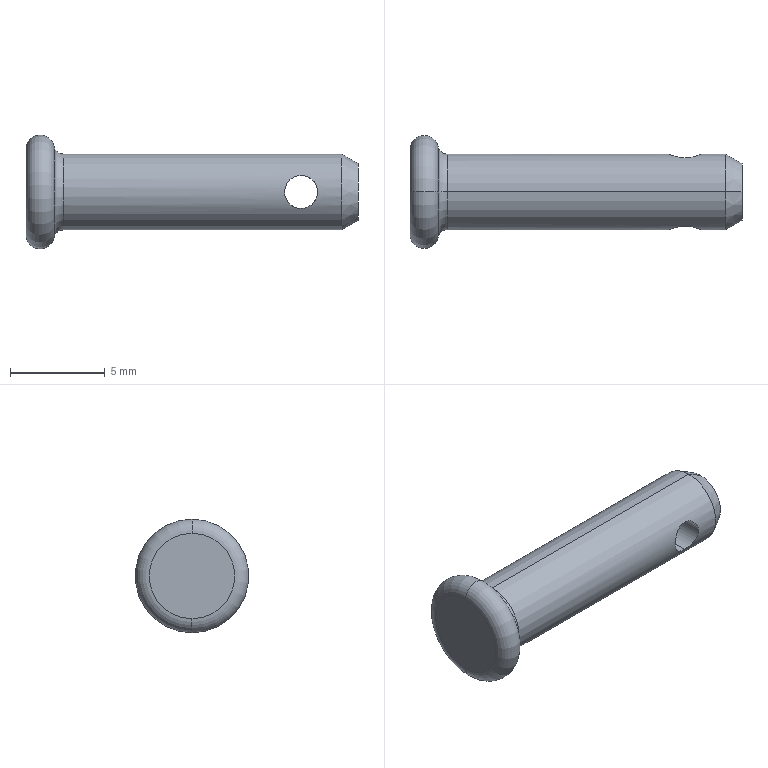Part | SolidWorks | features Chamfer 1, Cut 1, Fillet 1, Revolution 1 | 1 solid | 12 faces | box 17.5 x 6 x 6 mm | volume 227.981 mm3 | cylinder 4 | torus 4 | cone 2 | plane 2 | commonest cylinder face diameters 1.74 x2 4 x2
STEP:
#1=CARTESIAN_POINT('',(14.5,-1.801,-0.87));
#2=VERTEX_POINT('',#1);
#3=CARTESIAN_POINT('',(14.5,-1.801,0.87));
#4=VERTEX_POINT('',#3);
#5=CARTESIAN_POINT('',(14.5,-1.801,-0.87));
#6=CARTESIAN_POINT('',(14.385,-1.801,-0.87));
#7=CARTESIAN_POINT('',(14.27,-1.813,-0.8468));
#8=CARTESIAN_POINT('',(14.059,-1.851,-0.7588));
#9=CARTESIAN_POINT('',(13.964,-1.877,-0.6948));
#10=CARTESIAN_POINT('',(13.805,-1.929,-0.5353));
#11=CARTESIAN_POINT('',(13.741,-1.954,-0.4401));
#12=CARTESIAN_POINT('',(13.653,-1.99,-0.2304));
#13=CARTESIAN_POINT('',(13.63,-2.,-0.115));
#14=CARTESIAN_POINT('',(13.63,-2.,0.1145));
#15=CARTESIAN_POINT('',(13.653,-1.99,0.2302));
#16=CARTESIAN_POINT('',(13.741,-1.954,0.4402));
#17=CARTESIAN_POINT('',(13.805,-1.929,0.5355));
#18=CARTESIAN_POINT('',(14.045,-1.851,0.7751));
#19=CARTESIAN_POINT('',(14.267,-1.801,0.87));
#20=CARTESIAN_POINT('',(14.5,-1.801,0.87));
#21=B_SPLINE_CURVE_WITH_KNOTS('',3,(#5,#6,#7,#8,#9,#10,#11,#12,#13,#14,#15,#16,#17,#18,#19,#20),.UNSPECIFIED.,.F.,.F.,(4,2,2,2,2,2,2,4),(0.002755,0.003099,0.003443,0.003787,0.004131,0.004475,0.004819,0.005507),.UNSPECIFIED.);
#22=EDGE_CURVE('',#2,#4,#21,.T.);
#23=ORIENTED_EDGE('',*,*,#22,.F.);
#24=CARTESIAN_POINT('',(14.5,1.801,-0.87));
#25=VERTEX_POINT('',#24);
#26=CARTESIAN_POINT('',(14.5,-500.,-0.87));
#27=DIRECTION('',(0.,1.,0.));
#28=VECTOR('',#27,1000.);
#29=LINE('',#26,#28);
#30=EDGE_CURVE('',#2,#25,#29,.T.);
#31=ORIENTED_EDGE('',*,*,#30,.T.);
#32=CARTESIAN_POINT('',(14.5,1.801,0.87));
#33=VERTEX_POINT('',#32);
#34=CARTESIAN_POINT('',(14.5,1.801,0.87));
#35=CARTESIAN_POINT('',(14.383,1.801,0.87));
#36=CARTESIAN_POINT('',(14.269,1.813,0.8465));
#37=CARTESIAN_POINT('',(14.059,1.851,0.7588));
#38=CARTESIAN_POINT('',(13.964,1.877,0.6944));
#39=CARTESIAN_POINT('',(13.806,1.929,0.536));
#40=CARTESIAN_POINT('',(13.741,1.954,0.4402));
#41=CARTESIAN_POINT('',(13.654,1.989,0.2311));
#42=CARTESIAN_POINT('',(13.63,2.,0.1157));
#43=CARTESIAN_POINT('',(13.63,2.,-0.1148));
#44=CARTESIAN_POINT('',(13.653,1.99,-0.2298));
#45=CARTESIAN_POINT('',(13.742,1.954,-0.4417));
#46=CARTESIAN_POINT('',(13.806,1.928,-0.5366));
#47=CARTESIAN_POINT('',(13.965,1.877,-0.6952));
#48=CARTESIAN_POINT('',(14.061,1.851,-0.7594));
#49=CARTESIAN_POINT('',(14.269,1.813,-0.8465));
#50=CARTESIAN_POINT('',(14.385,1.801,-0.87));
#51=CARTESIAN_POINT('',(14.5,1.801,-0.87));
#52=B_SPLINE_CURVE_WITH_KNOTS('',3,(#34,#35,#36,#37,#38,#39,#40,#41,#42,#43,#44,#45,#46,#47,#48,#49,#50,#51),.UNSPECIFIED.,.F.,.F.,(4,2,2,2,2,2,2,2,4),(0.,0.0003443,0.0006887,0.001033,0.001377,0.001722,0.002066,0.00241,0.002755),.UNSPECIFIED.);
#53=EDGE_CURVE('',#33,#25,#52,.T.);
#54=ORIENTED_EDGE('',*,*,#53,.F.);
#55=CARTESIAN_POINT('',(14.5,-500.,0.87));
#56=DIRECTION('',(0.,1.,0.));
#57=VECTOR('',#56,1000.);
#58=LINE('',#55,#57);
#59=EDGE_CURVE('',#4,#33,#58,.T.);
#60=ORIENTED_EDGE('',*,*,#59,.F.);
#61=EDGE_LOOP('',(#23,#31,#54,#60));
#62=FACE_OUTER_BOUND('',#61,.T.);
#63=CARTESIAN_POINT('',(14.5,-500.,0.));
#64=DIRECTION('',(0.,1.,0.));
#65=DIRECTION('',(0.,0.,1.));
#66=AXIS2_PLACEMENT_3D('',#63,#64,#65);
#67=CYLINDRICAL_SURFACE('',#66,0.87);
#68=ADVANCED_FACE('',(#62),#67,.F.);
#69=CARTESIAN_POINT('',(17.5,0.,-1.5));
#70=VERTEX_POINT('',#69);
#71=CARTESIAN_POINT('',(17.5,0.,1.5));
#72=VERTEX_POINT('',#71);
#73=CARTESIAN_POINT('',(17.5,0.,0.));
#74=DIRECTION('',(1.,0.,0.));
#75=DIRECTION('',(0.,0.,1.));
#76=AXIS2_PLACEMENT_3D('',#73,#74,#75);
#77=CIRCLE('',#76,1.5);
#78=EDGE_CURVE('',#70,#72,#77,.T.);
#79=ORIENTED_EDGE('',*,*,#78,.F.);
#80=CARTESIAN_POINT('',(16.634,0.,-2.));
#81=VERTEX_POINT('',#80);
#82=CARTESIAN_POINT('',(16.634,0.,-2.));
#83=DIRECTION('',(-0.866,0.,-0.5));
#84=VECTOR('',#83,1000.);
#85=LINE('',#82,#84);
#86=EDGE_CURVE('',#70,#81,#85,.T.);
#87=ORIENTED_EDGE('',*,*,#86,.T.);
#88=CARTESIAN_POINT('',(16.634,0.,2.));
#89=VERTEX_POINT('',#88);
#90=CARTESIAN_POINT('',(16.634,0.,0.));
#91=DIRECTION('',(-1.,0.,0.));
#92=DIRECTION('',(0.,0.,1.));
#93=AXIS2_PLACEMENT_3D('',#90,#91,#92);
#94=CIRCLE('',#93,2.);
#95=EDGE_CURVE('',#89,#81,#94,.T.);
#96=ORIENTED_EDGE('',*,*,#95,.F.);
#97=CARTESIAN_POINT('',(16.634,0.,2.));
#98=DIRECTION('',(-0.866,0.,0.5));
#99=VECTOR('',#98,1000.);
#100=LINE('',#97,#99);
#101=EDGE_CURVE('',#72,#89,#100,.T.);
#102=ORIENTED_EDGE('',*,*,#101,.F.);
#103=EDGE_LOOP('',(#79,#87,#96,#102));
#104=FACE_OUTER_BOUND('',#103,.T.);
#105=CARTESIAN_POINT('',(16.634,0.,0.));
#106=DIRECTION('',(-1.,0.,0.));
#107=DIRECTION('',(0.,0.,1.));
#108=AXIS2_PLACEMENT_3D('',#105,#106,#107);
#109=CONICAL_SURFACE('',#108,2.,0.5236);
#110=ADVANCED_FACE('',(#104),#109,.T.);
#111=CARTESIAN_POINT('',(1.485,0.,-2.4));
#112=VERTEX_POINT('',#111);
#113=CARTESIAN_POINT('',(1.485,0.,2.4));
#114=VERTEX_POINT('',#113);
#115=CARTESIAN_POINT('',(1.485,0.,0.));
#116=DIRECTION('',(-1.,0.,0.));
#117=DIRECTION('',(0.,0.,1.));
#118=AXIS2_PLACEMENT_3D('',#115,#116,#117);
#119=CIRCLE('',#118,2.4);
#120=EDGE_CURVE('',#112,#114,#119,.T.);
#121=ORIENTED_EDGE('',*,*,#120,.F.);
#122=CARTESIAN_POINT('',(1.975,0.,-2.));
#123=VERTEX_POINT('',#122);
#124=CARTESIAN_POINT('',(1.975,0.,-2.5));
#125=DIRECTION('',(0.,1.,0.));
#126=DIRECTION('',(0.,0.,1.));
#127=AXIS2_PLACEMENT_3D('',#124,#125,#126);
#128=CIRCLE('',#127,0.5);
#129=EDGE_CURVE('',#112,#123,#128,.T.);
#130=ORIENTED_EDGE('',*,*,#129,.T.);
#131=CARTESIAN_POINT('',(1.975,0.,2.));
#132=VERTEX_POINT('',#131);
#133=CARTESIAN_POINT('',(1.975,0.,0.));
#134=DIRECTION('',(1.,0.,0.));
#135=DIRECTION('',(0.,0.,1.));
#136=AXIS2_PLACEMENT_3D('',#133,#134,#135);
#137=CIRCLE('',#136,2.);
#138=EDGE_CURVE('',#132,#123,#137,.T.);
#139=ORIENTED_EDGE('',*,*,#138,.F.);
#140=CARTESIAN_POINT('',(1.975,0.,2.5));
#141=DIRECTION('',(0.,-1.,0.));
#142=DIRECTION('',(0.,0.,-1.));
#143=AXIS2_PLACEMENT_3D('',#140,#141,#142);
#144=CIRCLE('',#143,0.5);
#145=EDGE_CURVE('',#114,#132,#144,.T.);
#146=ORIENTED_EDGE('',*,*,#145,.F.);
#147=EDGE_LOOP('',(#121,#130,#139,#146));
#148=FACE_OUTER_BOUND('',#147,.T.);
#149=CARTESIAN_POINT('',(1.975,0.,0.));
#150=DIRECTION('',(-1.,0.,0.));
#151=DIRECTION('',(0.,0.,1.));
#152=AXIS2_PLACEMENT_3D('',#149,#150,#151);
#153=TOROIDAL_SURFACE('',#152,2.5,0.5);
#154=ADVANCED_FACE('',(#148),#153,.F.);
#155=ORIENTED_EDGE('',*,*,#53,.T.);
#156=CARTESIAN_POINT('',(14.5,1.801,-0.87));
#157=CARTESIAN_POINT('',(14.615,1.801,-0.87));
#158=CARTESIAN_POINT('',(14.73,1.813,-0.8468));
#159=CARTESIAN_POINT('',(14.941,1.851,-0.7588));
#160=CARTESIAN_POINT('',(15.036,1.877,-0.6948));
#161=CARTESIAN_POINT('',(15.195,1.929,-0.5353));
#162=CARTESIAN_POINT('',(15.259,1.954,-0.4401));
#163=CARTESIAN_POINT('',(15.347,1.99,-0.2304));
#164=CARTESIAN_POINT('',(15.37,2.,-0.115));
#165=CARTESIAN_POINT('',(15.37,2.,0.1145));
#166=CARTESIAN_POINT('',(15.347,1.99,0.2302));
#167=CARTESIAN_POINT('',(15.259,1.954,0.4402));
#168=CARTESIAN_POINT('',(15.195,1.929,0.5355));
#169=CARTESIAN_POINT('',(14.955,1.851,0.7751));
#170=CARTESIAN_POINT('',(14.733,1.801,0.87));
#171=CARTESIAN_POINT('',(14.5,1.801,0.87));
#172=B_SPLINE_CURVE_WITH_KNOTS('',3,(#156,#157,#158,#159,#160,#161,#162,#163,#164,#165,#166,#167,#168,#169,#170,#171),.UNSPECIFIED.,.F.,.F.,(4,2,2,2,2,2,2,4),(0.002755,0.003099,0.003443,0.003787,0.004131,0.004475,0.004819,0.005507),.UNSPECIFIED.);
#173=EDGE_CURVE('',#25,#33,#172,.T.);
#174=ORIENTED_EDGE('',*,*,#173,.T.);
#175=EDGE_LOOP('',(#155,#174));
#176=FACE_BOUND('',#175,.T.);
#177=ORIENTED_EDGE('',*,*,#95,.T.);
#178=CARTESIAN_POINT('',(0.,0.,-2.));
#179=DIRECTION('',(-1.,0.,0.));
#180=VECTOR('',#179,1000.);
#181=LINE('',#178,#180);
#182=EDGE_CURVE('',#81,#123,#181,.T.);
#183=ORIENTED_EDGE('',*,*,#182,.T.);
#184=CARTESIAN_POINT('',(1.975,0.,0.));
#185=DIRECTION('',(1.,0.,0.));
#186=DIRECTION('',(0.,0.,1.));
#187=AXIS2_PLACEMENT_3D('',#184,#185,#186);
#188=CIRCLE('',#187,2.);
#189=EDGE_CURVE('',#123,#132,#188,.T.);
#190=ORIENTED_EDGE('',*,*,#189,.T.);
#191=CARTESIAN_POINT('',(0.,0.,2.));
#192=DIRECTION('',(-1.,0.,0.));
#193=VECTOR('',#192,1000.);
#194=LINE('',#191,#193);
#195=EDGE_CURVE('',#89,#132,#194,.T.);
#196=ORIENTED_EDGE('',*,*,#195,.F.);
#197=EDGE_LOOP('',(#177,#183,#190,#196));
#198=FACE_OUTER_BOUND('',#197,.T.);
#199=CARTESIAN_POINT('',(0.,0.,0.));
#200=DIRECTION('',(-1.,0.,0.));
#201=DIRECTION('',(0.,0.,1.));
#202=AXIS2_PLACEMENT_3D('',#199,#200,#201);
#203=CYLINDRICAL_SURFACE('',#202,2.);
#204=ADVANCED_FACE('',(#176,#198),#203,.T.);
#205=CARTESIAN_POINT('',(1.485,0.,0.));
#206=DIRECTION('',(-1.,0.,0.));
#207=DIRECTION('',(0.,0.,1.));
#208=AXIS2_PLACEMENT_3D('',#205,#206,#207);
#209=CIRCLE('',#208,2.4);
#210=EDGE_CURVE('',#114,#112,#209,.T.);
#211=ORIENTED_EDGE('',*,*,#210,.T.);
#212=CARTESIAN_POINT('',(0.,0.,-2.25));
#213=VERTEX_POINT('',#212);
#214=CARTESIAN_POINT('',(0.75,0.,-2.25));
#215=DIRECTION('',(0.,1.,0.));
#216=DIRECTION('',(0.,0.,1.));
#217=AXIS2_PLACEMENT_3D('',#214,#215,#216);
#218=CIRCLE('',#217,0.75);
#219=EDGE_CURVE('',#112,#213,#218,.T.);
#220=ORIENTED_EDGE('',*,*,#219,.T.);
#221=CARTESIAN_POINT('',(0.,0.,2.25));
#222=VERTEX_POINT('',#221);
#223=CARTESIAN_POINT('',(0.,0.,0.));
#224=DIRECTION('',(-1.,0.,0.));
#225=DIRECTION('',(0.,0.,1.));
#226=AXIS2_PLACEMENT_3D('',#223,#224,#225);
#227=CIRCLE('',#226,2.25);
#228=EDGE_CURVE('',#222,#213,#227,.T.);
#229=ORIENTED_EDGE('',*,*,#228,.F.);
#230=CARTESIAN_POINT('',(0.75,0.,2.25));
#231=DIRECTION('',(0.,-1.,0.));
#232=DIRECTION('',(0.,0.,-1.));
#233=AXIS2_PLACEMENT_3D('',#230,#231,#232);
#234=CIRCLE('',#233,0.75);
#235=EDGE_CURVE('',#114,#222,#234,.T.);
#236=ORIENTED_EDGE('',*,*,#235,.F.);
#237=EDGE_LOOP('',(#211,#220,#229,#236));
#238=FACE_OUTER_BOUND('',#237,.T.);
#239=CARTESIAN_POINT('',(0.75,0.,0.));
#240=DIRECTION('',(-1.,0.,0.));
#241=DIRECTION('',(0.,0.,1.));
#242=AXIS2_PLACEMENT_3D('',#239,#240,#241);
#243=TOROIDAL_SURFACE('',#242,2.25,0.75);
#244=ADVANCED_FACE('',(#238),#243,.T.);
#245=ORIENTED_EDGE('',*,*,#228,.T.);
#246=CARTESIAN_POINT('',(0.,0.,0.));
#247=DIRECTION('',(-1.,0.,0.));
#248=DIRECTION('',(0.,0.,1.));
#249=AXIS2_PLACEMENT_3D('',#246,#247,#248);
#250=CIRCLE('',#249,2.25);
#251=EDGE_CURVE('',#213,#222,#250,.T.);
#252=ORIENTED_EDGE('',*,*,#251,.T.);
#253=EDGE_LOOP('',(#245,#252));
#254=FACE_OUTER_BOUND('',#253,.T.);
#255=CARTESIAN_POINT('',(0.,0.,0.));
#256=DIRECTION('',(1.,0.,0.));
#257=DIRECTION('',(0.,0.,-1.));
#258=AXIS2_PLACEMENT_3D('',#255,#256,#257);
#259=PLANE('',#258);
#260=ADVANCED_FACE('',(#254),#259,.F.);
#261=ORIENTED_EDGE('',*,*,#219,.F.);
#262=ORIENTED_EDGE('',*,*,#120,.T.);
#263=ORIENTED_EDGE('',*,*,#235,.T.);
#264=ORIENTED_EDGE('',*,*,#251,.F.);
#265=EDGE_LOOP('',(#261,#262,#263,#264));
#266=FACE_OUTER_BOUND('',#265,.T.);
#267=CARTESIAN_POINT('',(0.75,0.,0.));
#268=DIRECTION('',(-1.,0.,0.));
#269=DIRECTION('',(0.,0.,1.));
#270=AXIS2_PLACEMENT_3D('',#267,#268,#269);
#271=TOROIDAL_SURFACE('',#270,2.25,0.75);
#272=ADVANCED_FACE('',(#266),#271,.T.);
#273=ORIENTED_EDGE('',*,*,#182,.F.);
#274=CARTESIAN_POINT('',(16.634,0.,0.));
#275=DIRECTION('',(-1.,0.,0.));
#276=DIRECTION('',(0.,0.,1.));
#277=AXIS2_PLACEMENT_3D('',#274,#275,#276);
#278=CIRCLE('',#277,2.);
#279=EDGE_CURVE('',#81,#89,#278,.T.);
#280=ORIENTED_EDGE('',*,*,#279,.T.);
#281=ORIENTED_EDGE('',*,*,#195,.T.);
#282=ORIENTED_EDGE('',*,*,#138,.T.);
#283=EDGE_LOOP('',(#273,#280,#281,#282));
#284=FACE_OUTER_BOUND('',#283,.T.);
#285=CARTESIAN_POINT('',(14.5,-1.801,0.87));
#286=CARTESIAN_POINT('',(14.617,-1.801,0.87));
#287=CARTESIAN_POINT('',(14.731,-1.813,0.8465));
#288=CARTESIAN_POINT('',(14.941,-1.851,0.7588));
#289=CARTESIAN_POINT('',(15.036,-1.877,0.6944));
#290=CARTESIAN_POINT('',(15.194,-1.929,0.536));
#291=CARTESIAN_POINT('',(15.259,-1.954,0.4402));
#292=CARTESIAN_POINT('',(15.346,-1.989,0.2311));
#293=CARTESIAN_POINT('',(15.37,-2.,0.1157));
#294=CARTESIAN_POINT('',(15.37,-2.,-0.1148));
#295=CARTESIAN_POINT('',(15.347,-1.99,-0.2298));
#296=CARTESIAN_POINT('',(15.258,-1.954,-0.4417));
#297=CARTESIAN_POINT('',(15.194,-1.928,-0.5366));
#298=CARTESIAN_POINT('',(15.035,-1.877,-0.6952));
#299=CARTESIAN_POINT('',(14.939,-1.851,-0.7594));
#300=CARTESIAN_POINT('',(14.731,-1.813,-0.8465));
#301=CARTESIAN_POINT('',(14.615,-1.801,-0.87));
#302=CARTESIAN_POINT('',(14.5,-1.801,-0.87));
#303=B_SPLINE_CURVE_WITH_KNOTS('',3,(#285,#286,#287,#288,#289,#290,#291,#292,#293,#294,#295,#296,#297,#298,#299,#300,#301,#302),.UNSPECIFIED.,.F.,.F.,(4,2,2,2,2,2,2,2,4),(0.,0.0003443,0.0006887,0.001033,0.001377,0.001722,0.002066,0.00241,0.002755),.UNSPECIFIED.);
#304=EDGE_CURVE('',#4,#2,#303,.T.);
#305=ORIENTED_EDGE('',*,*,#304,.T.);
#306=ORIENTED_EDGE('',*,*,#22,.T.);
#307=EDGE_LOOP('',(#305,#306));
#308=FACE_BOUND('',#307,.T.);
#309=CARTESIAN_POINT('',(0.,0.,0.));
#310=DIRECTION('',(-1.,0.,0.));
#311=DIRECTION('',(0.,0.,1.));
#312=AXIS2_PLACEMENT_3D('',#309,#310,#311);
#313=CYLINDRICAL_SURFACE('',#312,2.);
#314=ADVANCED_FACE('',(#284,#308),#313,.T.);
#315=CARTESIAN_POINT('',(17.5,0.,0.));
#316=DIRECTION('',(1.,0.,0.));
#317=DIRECTION('',(0.,0.,1.));
#318=AXIS2_PLACEMENT_3D('',#315,#316,#317);
#319=CIRCLE('',#318,1.5);
#320=EDGE_CURVE('',#72,#70,#319,.T.);
#321=ORIENTED_EDGE('',*,*,#320,.T.);
#322=ORIENTED_EDGE('',*,*,#78,.T.);
#323=EDGE_LOOP('',(#321,#322));
#324=FACE_OUTER_BOUND('',#323,.T.);
#325=CARTESIAN_POINT('',(17.5,2.,0.));
#326=DIRECTION('',(-1.,0.,0.));
#327=DIRECTION('',(0.,0.,1.));
#328=AXIS2_PLACEMENT_3D('',#325,#326,#327);
#329=PLANE('',#328);
#330=ADVANCED_FACE('',(#324),#329,.F.);
#331=ORIENTED_EDGE('',*,*,#129,.F.);
#332=ORIENTED_EDGE('',*,*,#210,.F.);
#333=ORIENTED_EDGE('',*,*,#145,.T.);
#334=ORIENTED_EDGE('',*,*,#189,.F.);
#335=EDGE_LOOP('',(#331,#332,#333,#334));
#336=FACE_OUTER_BOUND('',#335,.T.);
#337=CARTESIAN_POINT('',(1.975,0.,0.));
#338=DIRECTION('',(-1.,0.,0.));
#339=DIRECTION('',(0.,0.,1.));
#340=AXIS2_PLACEMENT_3D('',#337,#338,#339);
#341=TOROIDAL_SURFACE('',#340,2.5,0.5);
#342=ADVANCED_FACE('',(#336),#341,.F.);
#343=ORIENTED_EDGE('',*,*,#86,.F.);
#344=ORIENTED_EDGE('',*,*,#320,.F.);
#345=ORIENTED_EDGE('',*,*,#101,.T.);
#346=ORIENTED_EDGE('',*,*,#279,.F.);
#347=EDGE_LOOP('',(#343,#344,#345,#346));
#348=FACE_OUTER_BOUND('',#347,.T.);
#349=CARTESIAN_POINT('',(16.634,0.,0.));
#350=DIRECTION('',(-1.,0.,0.));
#351=DIRECTION('',(0.,0.,1.));
#352=AXIS2_PLACEMENT_3D('',#349,#350,#351);
#353=CONICAL_SURFACE('',#352,2.,0.5236);
#354=ADVANCED_FACE('',(#348),#353,.T.);
#355=ORIENTED_EDGE('',*,*,#30,.F.);
#356=ORIENTED_EDGE('',*,*,#304,.F.);
#357=ORIENTED_EDGE('',*,*,#59,.T.);
#358=ORIENTED_EDGE('',*,*,#173,.F.);
#359=EDGE_LOOP('',(#355,#356,#357,#358));
#360=FACE_OUTER_BOUND('',#359,.T.);
#361=CARTESIAN_POINT('',(14.5,-500.,0.));
#362=DIRECTION('',(0.,1.,0.));
#363=DIRECTION('',(0.,0.,1.));
#364=AXIS2_PLACEMENT_3D('',#361,#362,#363);
#365=CYLINDRICAL_SURFACE('',#364,0.87);
#366=ADVANCED_FACE('',(#360),#365,.F.);
#367=CLOSED_SHELL('',(#68,#110,#154,#204,#244,#260,#272,#314,#330,#342,#354,#366));
#368=MANIFOLD_SOLID_BREP('',#367);
#369=CARTESIAN_POINT('',(0.,0.,0.));
#370=DIRECTION('',(0.,0.,1.));
#371=DIRECTION('',(1.,0.,0.));
#372=AXIS2_PLACEMENT_3D('',#369,#370,#371);
#373=(LENGTH_UNIT()NAMED_UNIT(*)SI_UNIT(.MILLI.,.METRE.));
#374=UNCERTAINTY_MEASURE_WITH_UNIT(LENGTH_MEASURE(0.00001),#373,'','');
#375=(NAMED_UNIT(*)PLANE_ANGLE_UNIT()SI_UNIT($,.RADIAN.));
#376=(NAMED_UNIT(*)SI_UNIT($,.STERADIAN.)SOLID_ANGLE_UNIT());
#377=(GEOMETRIC_REPRESENTATION_CONTEXT(3)GLOBAL_UNCERTAINTY_ASSIGNED_CONTEXT((#374))GLOBAL_UNIT_ASSIGNED_CONTEXT((#373,#375,#376))REPRESENTATION_CONTEXT('',''));
#378=ADVANCED_BREP_SHAPE_REPRESENTATION('',(#368,#372),#377);